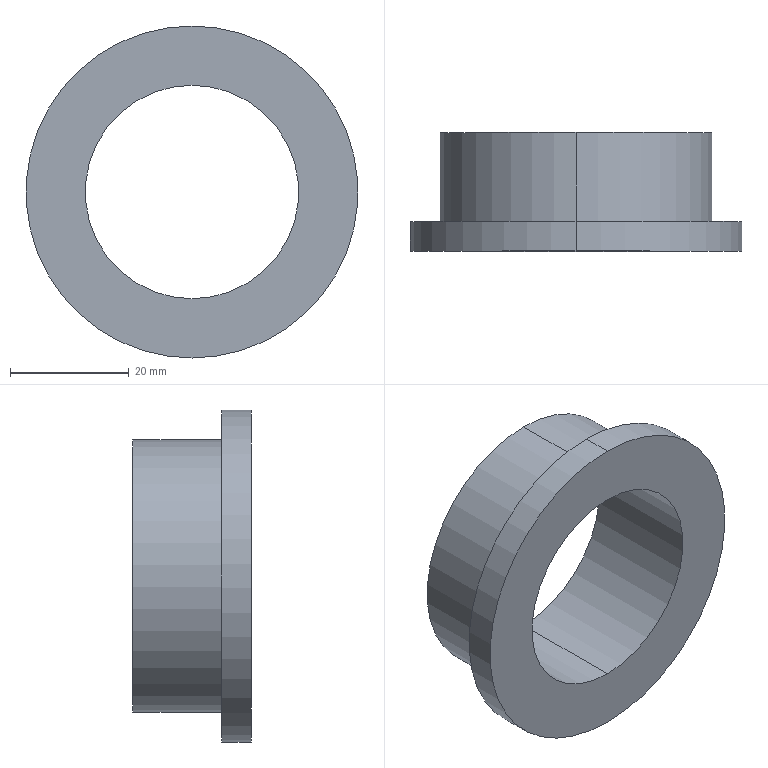Part | SolidWorks | features Extrusion 1, ICE 1 | 1 solid | 9 faces | box 56 x 20 x 56 mm | volume 16886 mm3 | cylinder 6 | plane 3 | commonest cylinder face diameters 36 x2 46 x2 56 x2
STEP:
#1=CARTESIAN_POINT('',(0.,20.,23.));
#2=VERTEX_POINT('',#1);
#3=CARTESIAN_POINT('',(0.,20.,-23.));
#4=VERTEX_POINT('',#3);
#5=CARTESIAN_POINT('',(0.,20.,0.));
#6=DIRECTION('',(0.,1.,0.));
#7=DIRECTION('',(0.,0.,1.));
#8=AXIS2_PLACEMENT_3D('',#5,#6,#7);
#9=CIRCLE('',#8,23.);
#10=EDGE_CURVE('',#2,#4,#9,.T.);
#11=ORIENTED_EDGE('',*,*,#10,.F.);
#12=CARTESIAN_POINT('',(0.,5.,23.));
#13=VERTEX_POINT('',#12);
#14=CARTESIAN_POINT('',(0.,20.,23.));
#15=DIRECTION('',(0.,-1.,0.));
#16=VECTOR('',#15,1000.);
#17=LINE('',#14,#16);
#18=EDGE_CURVE('',#2,#13,#17,.T.);
#19=ORIENTED_EDGE('',*,*,#18,.T.);
#20=CARTESIAN_POINT('',(0.,5.,-23.));
#21=VERTEX_POINT('',#20);
#22=CARTESIAN_POINT('',(0.,5.,0.));
#23=DIRECTION('',(0.,1.,0.));
#24=DIRECTION('',(0.,0.,1.));
#25=AXIS2_PLACEMENT_3D('',#22,#23,#24);
#26=CIRCLE('',#25,23.);
#27=EDGE_CURVE('',#13,#21,#26,.T.);
#28=ORIENTED_EDGE('',*,*,#27,.T.);
#29=CARTESIAN_POINT('',(0.,20.,-23.));
#30=DIRECTION('',(0.,-1.,0.));
#31=VECTOR('',#30,1000.);
#32=LINE('',#29,#31);
#33=EDGE_CURVE('',#4,#21,#32,.T.);
#34=ORIENTED_EDGE('',*,*,#33,.F.);
#35=EDGE_LOOP('',(#11,#19,#28,#34));
#36=FACE_OUTER_BOUND('',#35,.T.);
#37=CARTESIAN_POINT('',(0.,20.,0.));
#38=DIRECTION('',(0.,-1.,0.));
#39=DIRECTION('',(0.,0.,-1.));
#40=AXIS2_PLACEMENT_3D('',#37,#38,#39);
#41=CYLINDRICAL_SURFACE('',#40,23.);
#42=ADVANCED_FACE('',(#36),#41,.T.);
#43=CARTESIAN_POINT('',(0.,20.,-18.));
#44=VERTEX_POINT('',#43);
#45=CARTESIAN_POINT('',(0.,20.,18.));
#46=VERTEX_POINT('',#45);
#47=CARTESIAN_POINT('',(0.,20.,0.));
#48=DIRECTION('',(0.,1.,0.));
#49=DIRECTION('',(0.,0.,1.));
#50=AXIS2_PLACEMENT_3D('',#47,#48,#49);
#51=CIRCLE('',#50,18.);
#52=EDGE_CURVE('',#44,#46,#51,.T.);
#53=ORIENTED_EDGE('',*,*,#52,.T.);
#54=CARTESIAN_POINT('',(0.,0.,18.));
#55=VERTEX_POINT('',#54);
#56=CARTESIAN_POINT('',(0.,5.,18.));
#57=DIRECTION('',(0.,-1.,0.));
#58=VECTOR('',#57,1000.);
#59=LINE('',#56,#58);
#60=EDGE_CURVE('',#46,#55,#59,.T.);
#61=ORIENTED_EDGE('',*,*,#60,.T.);
#62=CARTESIAN_POINT('',(0.,0.,-18.));
#63=VERTEX_POINT('',#62);
#64=CARTESIAN_POINT('',(0.,0.,0.));
#65=DIRECTION('',(0.,1.,0.));
#66=DIRECTION('',(0.,0.,1.));
#67=AXIS2_PLACEMENT_3D('',#64,#65,#66);
#68=CIRCLE('',#67,18.);
#69=EDGE_CURVE('',#63,#55,#68,.T.);
#70=ORIENTED_EDGE('',*,*,#69,.F.);
#71=CARTESIAN_POINT('',(0.,5.,-18.));
#72=DIRECTION('',(0.,-1.,0.));
#73=VECTOR('',#72,1000.);
#74=LINE('',#71,#73);
#75=EDGE_CURVE('',#44,#63,#74,.T.);
#76=ORIENTED_EDGE('',*,*,#75,.F.);
#77=EDGE_LOOP('',(#53,#61,#70,#76));
#78=FACE_OUTER_BOUND('',#77,.T.);
#79=CARTESIAN_POINT('',(0.,5.,0.));
#80=DIRECTION('',(0.,-1.,0.));
#81=DIRECTION('',(0.,0.,-1.));
#82=AXIS2_PLACEMENT_3D('',#79,#80,#81);
#83=CYLINDRICAL_SURFACE('',#82,18.);
#84=ADVANCED_FACE('',(#78),#83,.F.);
#85=CARTESIAN_POINT('',(0.,5.,28.));
#86=VERTEX_POINT('',#85);
#87=CARTESIAN_POINT('',(0.,5.,-28.));
#88=VERTEX_POINT('',#87);
#89=CARTESIAN_POINT('',(0.,5.,0.));
#90=DIRECTION('',(0.,1.,0.));
#91=DIRECTION('',(0.,0.,1.));
#92=AXIS2_PLACEMENT_3D('',#89,#90,#91);
#93=CIRCLE('',#92,28.);
#94=EDGE_CURVE('',#86,#88,#93,.T.);
#95=ORIENTED_EDGE('',*,*,#94,.F.);
#96=CARTESIAN_POINT('',(0.,0.,28.));
#97=VERTEX_POINT('',#96);
#98=CARTESIAN_POINT('',(0.,5.,28.));
#99=DIRECTION('',(0.,-1.,0.));
#100=VECTOR('',#99,1000.);
#101=LINE('',#98,#100);
#102=EDGE_CURVE('',#86,#97,#101,.T.);
#103=ORIENTED_EDGE('',*,*,#102,.T.);
#104=CARTESIAN_POINT('',(0.,0.,-28.));
#105=VERTEX_POINT('',#104);
#106=CARTESIAN_POINT('',(0.,0.,0.));
#107=DIRECTION('',(0.,1.,0.));
#108=DIRECTION('',(0.,0.,1.));
#109=AXIS2_PLACEMENT_3D('',#106,#107,#108);
#110=CIRCLE('',#109,28.);
#111=EDGE_CURVE('',#97,#105,#110,.T.);
#112=ORIENTED_EDGE('',*,*,#111,.T.);
#113=CARTESIAN_POINT('',(0.,5.,-28.));
#114=DIRECTION('',(0.,-1.,0.));
#115=VECTOR('',#114,1000.);
#116=LINE('',#113,#115);
#117=EDGE_CURVE('',#88,#105,#116,.T.);
#118=ORIENTED_EDGE('',*,*,#117,.F.);
#119=EDGE_LOOP('',(#95,#103,#112,#118));
#120=FACE_OUTER_BOUND('',#119,.T.);
#121=CARTESIAN_POINT('',(0.,5.,0.));
#122=DIRECTION('',(0.,-1.,0.));
#123=DIRECTION('',(0.,0.,-1.));
#124=AXIS2_PLACEMENT_3D('',#121,#122,#123);
#125=CYLINDRICAL_SURFACE('',#124,28.);
#126=ADVANCED_FACE('',(#120),#125,.T.);
#127=CARTESIAN_POINT('',(0.,5.,0.));
#128=DIRECTION('',(0.,1.,0.));
#129=DIRECTION('',(0.,0.,1.));
#130=AXIS2_PLACEMENT_3D('',#127,#128,#129);
#131=CIRCLE('',#130,28.);
#132=EDGE_CURVE('',#88,#86,#131,.T.);
#133=ORIENTED_EDGE('',*,*,#132,.T.);
#134=ORIENTED_EDGE('',*,*,#94,.T.);
#135=EDGE_LOOP('',(#133,#134));
#136=FACE_OUTER_BOUND('',#135,.T.);
#137=CARTESIAN_POINT('',(0.,5.,0.));
#138=DIRECTION('',(0.,1.,0.));
#139=DIRECTION('',(0.,0.,1.));
#140=AXIS2_PLACEMENT_3D('',#137,#138,#139);
#141=CIRCLE('',#140,23.);
#142=EDGE_CURVE('',#21,#13,#141,.T.);
#143=ORIENTED_EDGE('',*,*,#142,.F.);
#144=ORIENTED_EDGE('',*,*,#27,.F.);
#145=EDGE_LOOP('',(#143,#144));
#146=FACE_BOUND('',#145,.T.);
#147=CARTESIAN_POINT('',(0.,5.,0.));
#148=DIRECTION('',(0.,1.,0.));
#149=DIRECTION('',(0.,0.,1.));
#150=AXIS2_PLACEMENT_3D('',#147,#148,#149);
#151=PLANE('',#150);
#152=ADVANCED_FACE('',(#136,#146),#151,.T.);
#153=CARTESIAN_POINT('',(0.,0.,0.));
#154=DIRECTION('',(0.,1.,0.));
#155=DIRECTION('',(0.,0.,1.));
#156=AXIS2_PLACEMENT_3D('',#153,#154,#155);
#157=CIRCLE('',#156,28.);
#158=EDGE_CURVE('',#105,#97,#157,.T.);
#159=ORIENTED_EDGE('',*,*,#158,.F.);
#160=ORIENTED_EDGE('',*,*,#111,.F.);
#161=EDGE_LOOP('',(#159,#160));
#162=FACE_OUTER_BOUND('',#161,.T.);
#163=ORIENTED_EDGE('',*,*,#69,.T.);
#164=CARTESIAN_POINT('',(0.,0.,0.));
#165=DIRECTION('',(0.,1.,0.));
#166=DIRECTION('',(0.,0.,1.));
#167=AXIS2_PLACEMENT_3D('',#164,#165,#166);
#168=CIRCLE('',#167,18.);
#169=EDGE_CURVE('',#55,#63,#168,.T.);
#170=ORIENTED_EDGE('',*,*,#169,.T.);
#171=EDGE_LOOP('',(#163,#170));
#172=FACE_BOUND('',#171,.T.);
#173=CARTESIAN_POINT('',(0.,0.,0.));
#174=DIRECTION('',(0.,1.,0.));
#175=DIRECTION('',(0.,0.,1.));
#176=AXIS2_PLACEMENT_3D('',#173,#174,#175);
#177=PLANE('',#176);
#178=ADVANCED_FACE('',(#162,#172),#177,.F.);
#179=ORIENTED_EDGE('',*,*,#102,.F.);
#180=ORIENTED_EDGE('',*,*,#132,.F.);
#181=ORIENTED_EDGE('',*,*,#117,.T.);
#182=ORIENTED_EDGE('',*,*,#158,.T.);
#183=EDGE_LOOP('',(#179,#180,#181,#182));
#184=FACE_OUTER_BOUND('',#183,.T.);
#185=CARTESIAN_POINT('',(0.,5.,0.));
#186=DIRECTION('',(0.,-1.,0.));
#187=DIRECTION('',(0.,0.,-1.));
#188=AXIS2_PLACEMENT_3D('',#185,#186,#187);
#189=CYLINDRICAL_SURFACE('',#188,28.);
#190=ADVANCED_FACE('',(#184),#189,.T.);
#191=ORIENTED_EDGE('',*,*,#60,.F.);
#192=CARTESIAN_POINT('',(0.,20.,0.));
#193=DIRECTION('',(0.,1.,0.));
#194=DIRECTION('',(0.,0.,1.));
#195=AXIS2_PLACEMENT_3D('',#192,#193,#194);
#196=CIRCLE('',#195,18.);
#197=EDGE_CURVE('',#46,#44,#196,.T.);
#198=ORIENTED_EDGE('',*,*,#197,.T.);
#199=ORIENTED_EDGE('',*,*,#75,.T.);
#200=ORIENTED_EDGE('',*,*,#169,.F.);
#201=EDGE_LOOP('',(#191,#198,#199,#200));
#202=FACE_OUTER_BOUND('',#201,.T.);
#203=CARTESIAN_POINT('',(0.,5.,0.));
#204=DIRECTION('',(0.,-1.,0.));
#205=DIRECTION('',(0.,0.,-1.));
#206=AXIS2_PLACEMENT_3D('',#203,#204,#205);
#207=CYLINDRICAL_SURFACE('',#206,18.);
#208=ADVANCED_FACE('',(#202),#207,.F.);
#209=CARTESIAN_POINT('',(0.,20.,0.));
#210=DIRECTION('',(0.,1.,0.));
#211=DIRECTION('',(0.,0.,1.));
#212=AXIS2_PLACEMENT_3D('',#209,#210,#211);
#213=CIRCLE('',#212,23.);
#214=EDGE_CURVE('',#4,#2,#213,.T.);
#215=ORIENTED_EDGE('',*,*,#214,.T.);
#216=ORIENTED_EDGE('',*,*,#10,.T.);
#217=EDGE_LOOP('',(#215,#216));
#218=FACE_OUTER_BOUND('',#217,.T.);
#219=ORIENTED_EDGE('',*,*,#52,.F.);
#220=ORIENTED_EDGE('',*,*,#197,.F.);
#221=EDGE_LOOP('',(#219,#220));
#222=FACE_BOUND('',#221,.T.);
#223=CARTESIAN_POINT('',(0.,20.,0.));
#224=DIRECTION('',(0.,1.,0.));
#225=DIRECTION('',(0.,0.,1.));
#226=AXIS2_PLACEMENT_3D('',#223,#224,#225);
#227=PLANE('',#226);
#228=ADVANCED_FACE('',(#218,#222),#227,.T.);
#229=ORIENTED_EDGE('',*,*,#18,.F.);
#230=ORIENTED_EDGE('',*,*,#214,.F.);
#231=ORIENTED_EDGE('',*,*,#33,.T.);
#232=ORIENTED_EDGE('',*,*,#142,.T.);
#233=EDGE_LOOP('',(#229,#230,#231,#232));
#234=FACE_OUTER_BOUND('',#233,.T.);
#235=CARTESIAN_POINT('',(0.,20.,0.));
#236=DIRECTION('',(0.,-1.,0.));
#237=DIRECTION('',(0.,0.,-1.));
#238=AXIS2_PLACEMENT_3D('',#235,#236,#237);
#239=CYLINDRICAL_SURFACE('',#238,23.);
#240=ADVANCED_FACE('',(#234),#239,.T.);
#241=CLOSED_SHELL('',(#42,#84,#126,#152,#178,#190,#208,#228,#240));
#242=MANIFOLD_SOLID_BREP('',#241);
#243=CARTESIAN_POINT('',(0.,0.,0.));
#244=DIRECTION('',(0.,0.,1.));
#245=DIRECTION('',(1.,0.,0.));
#246=AXIS2_PLACEMENT_3D('',#243,#244,#245);
#247=(LENGTH_UNIT()NAMED_UNIT(*)SI_UNIT(.MILLI.,.METRE.));
#248=UNCERTAINTY_MEASURE_WITH_UNIT(LENGTH_MEASURE(0.00001),#247,'','');
#249=(NAMED_UNIT(*)PLANE_ANGLE_UNIT()SI_UNIT($,.RADIAN.));
#250=(NAMED_UNIT(*)SI_UNIT($,.STERADIAN.)SOLID_ANGLE_UNIT());
#251=(GEOMETRIC_REPRESENTATION_CONTEXT(3)GLOBAL_UNCERTAINTY_ASSIGNED_CONTEXT((#248))GLOBAL_UNIT_ASSIGNED_CONTEXT((#247,#249,#250))REPRESENTATION_CONTEXT('',''));
#252=ADVANCED_BREP_SHAPE_REPRESENTATION('',(#242,#246),#251);